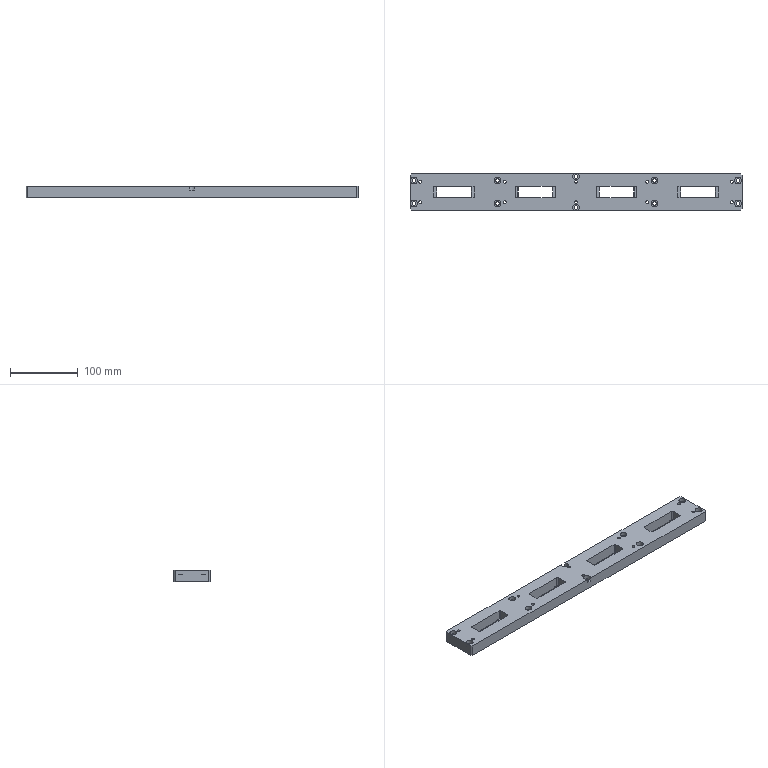NC program | NX | posted with a generic post | part box 490 x 54 x 17 mm
Lines 1858 to 2864 of 8955:
(ZLEVEL_PROFILE_COPY , TOOL : D4)
N3672 T11 M6
N3674 G54
N3676 G17 G0 G90 X449.641 Y-33.2 S8500 M3
N3678 G43 Z30. H11
N3680 Z1.108
N3682 G94 G1 Z-0.392 F1000.
N3684 X449.757 Y-33.4
N3686 G3 X450.103 Y-33.6 R0.4
N3688 G1 X453. F1500.
N3690 Y-30.703
N3692 G3 X452.8 Y-30.357 R0.4
N3694 G1 X452.6 Y-30.241
N3696 Z1.108
N3698 G0 X449.641 Y-33.2 Z0.716
N3700 G1 Z-0.784 F1000.
N3702 X449.757 Y-33.4
N3704 G3 X450.103 Y-33.6 R0.4
N3706 G1 X453. F1500.
N3708 Y-30.703
N3710 G3 X452.8 Y-30.357 R0.4
N3712 G1 X452.6 Y-30.241
N3714 Z0.716
N3716 G0 X449.641 Y-33.2 Z0.324
N3718 G1 Z-1.176 F1000.
N3720 X449.757 Y-33.4
N3722 G3 X450.103 Y-33.6 R0.4
N3724 G1 X453. F1500.
N3726 Y-30.703
N3728 G3 X452.8 Y-30.357 R0.4
N3730 G1 X452.6 Y-30.241
N3732 Z0.324
N3734 G0 X449.641 Y-33.2 Z-0.068
N3736 G1 Z-1.568 F1000.
N3738 X449.757 Y-33.4
N3740 G3 X450.103 Y-33.6 R0.4
N3742 G1 X453. F1500.
N3744 Y-30.703
N3746 G3 X452.8 Y-30.357 R0.4
N3748 G1 X452.6 Y-30.241
N3750 Z-0.068
N3752 G0 X449.641 Y-33.2 Z-0.459
N3754 G1 Z-1.959 F1000.
N3756 X449.757 Y-33.4
N3758 G3 X450.103 Y-33.6 R0.4
N3760 G1 X453. F1500.
N3762 Y-30.703
N3764 G3 X452.8 Y-30.357 R0.4
N3766 G1 X452.6 Y-30.241
N3768 Z-0.459
N3770 G0 X449.641 Y-33.2 Z-0.851
N3772 G1 Z-2.351 F1000.
N3774 X449.757 Y-33.4
N3776 G3 X450.103 Y-33.6 R0.4
N3778 G1 X453. F1500.
N3780 Y-30.703
N3782 G3 X452.8 Y-30.357 R0.4
N3784 G1 X452.6 Y-30.241
N3786 Z-0.851
N3788 G0 X449.641 Y-33.2 Z-1.243
N3790 G1 Z-2.743 F1000.
N3792 X449.757 Y-33.4
N3794 G3 X450.103 Y-33.6 R0.4
N3796 G1 X453. F1500.
N3798 Y-30.703
N3800 G3 X452.8 Y-30.357 R0.4
N3802 G1 X452.6 Y-30.241
N3804 Z-1.243
N3806 G0 X449.641 Y-33.2 Z-1.635
N3808 G1 Z-3.135 F1000.
N3810 X449.757 Y-33.4
N3812 G3 X450.103 Y-33.6 R0.4
N3814 G1 X453. F1500.
N3816 Y-30.703
N3818 G3 X452.8 Y-30.357 R0.4
N3820 G1 X452.6 Y-30.241
N3822 Z-1.635
N3824 G0 X449.641 Y-33.2 Z-2.027
N3826 G1 Z-3.527 F1000.
N3828 X449.757 Y-33.4
N3830 G3 X450.103 Y-33.6 R0.4
N3832 G1 X453. F1500.
N3834 Y-30.703
N3836 G3 X452.8 Y-30.357 R0.4
N3838 G1 X452.6 Y-30.241
N3840 Z-2.027
N3842 G0 X449.641 Y-33.2 Z-2.419
N3844 G1 Z-3.919 F1000.
N3846 X449.757 Y-33.4
N3848 G3 X450.103 Y-33.6 R0.4
N3850 G1 X453. F1500.
N3852 Y-30.703
N3854 G3 X452.8 Y-30.357 R0.4
N3856 G1 X452.6 Y-30.241
N3858 Z-2.419
N3860 G0 X449.641 Y-33.2 Z-2.811
N3862 G1 Z-4.311 F1000.
N3864 X449.757 Y-33.4
N3866 G3 X450.103 Y-33.6 R0.4
N3868 G1 X453. F1500.
N3870 Y-30.703
N3872 G3 X452.8 Y-30.357 R0.4
N3874 G1 X452.6 Y-30.241
N3876 Z-2.811
N3878 G0 X449.641 Y-33.2 Z-3.203
N3880 G1 Z-4.703 F1000.
N3882 X449.757 Y-33.4
N3884 G3 X450.103 Y-33.6 R0.4
N3886 G1 X453. F1500.
N3888 Y-30.703
N3890 G3 X452.8 Y-30.357 R0.4
N3892 G1 X452.6 Y-30.241
N3894 Z-3.203
N3896 G0 X449.641 Y-33.2 Z-3.595
N3898 G1 Z-5.095 F1000.
N3900 X449.757 Y-33.4
N3902 G3 X450.103 Y-33.6 R0.4
N3904 G1 X453. F1500.
N3906 Y-30.703
N3908 G3 X452.8 Y-30.357 R0.4
N3910 G1 X452.6 Y-30.241
N3912 Z-3.595
N3914 G0 X449.641 Y-33.2 Z-3.986
N3916 G1 Z-5.486 F1000.
N3918 X449.757 Y-33.4
N3920 G3 X450.103 Y-33.6 R0.4
N3922 G1 X453. F1500.
N3924 Y-30.703
N3926 G3 X452.8 Y-30.357 R0.4
N3928 G1 X452.6 Y-30.241
N3930 Z-3.986
N3932 G0 X449.641 Y-33.2 Z-4.378
N3934 G1 Z-5.878 F1000.
N3936 X449.757 Y-33.4
N3938 G3 X450.103 Y-33.6 R0.4
N3940 G1 X453. F1500.
N3942 Y-30.703
N3944 G3 X452.8 Y-30.357 R0.4
N3946 G1 X452.6 Y-30.241
N3948 Z-4.378
N3950 G0 X449.641 Y-33.2 Z-4.77
N3952 G1 Z-6.27 F1000.
N3954 X449.757 Y-33.4
N3956 G3 X450.103 Y-33.6 R0.4
N3958 G1 X453. F1500.
N3960 Y-30.703
N3962 G3 X452.8 Y-30.357 R0.4
N3964 G1 X452.6 Y-30.241
N3966 Z-4.77
N3968 G0 X449.641 Y-33.2 Z-5.162
N3970 G1 Z-6.662 F1000.
N3972 X449.757 Y-33.4
N3974 G3 X450.103 Y-33.6 R0.4
N3976 G1 X453. F1500.
N3978 Y-30.703
N3980 G3 X452.8 Y-30.357 R0.4
N3982 G1 X452.6 Y-30.241
N3984 Z-5.162
N3986 G0 X449.641 Y-33.2 Z-5.554
N3988 G1 Z-7.054 F1000.
N3990 X449.757 Y-33.4
N3992 G3 X450.103 Y-33.6 R0.4
N3994 G1 X453. F1500.
N3996 Y-30.703
N3998 G3 X452.8 Y-30.357 R0.4
N4000 G1 X452.6 Y-30.241
N4002 Z-5.554
N4004 G0 X449.641 Y-33.2 Z-5.946
N4006 G1 Z-7.446 F1000.
N4008 X449.757 Y-33.4
N4010 G3 X450.103 Y-33.6 R0.4
N4012 G1 X453. F1500.
N4014 Y-30.703
N4016 G3 X452.8 Y-30.357 R0.4
N4018 G1 X452.6 Y-30.241
N4020 Z-5.946
N4022 G0 X449.641 Y-33.2 Z-6.338
N4024 G1 Z-7.838 F1000.
N4026 X449.757 Y-33.4
N4028 G3 X450.103 Y-33.6 R0.4
N4030 G1 X453. F1500.
N4032 Y-30.703
N4034 G3 X452.8 Y-30.357 R0.4
N4036 G1 X452.6 Y-30.241
N4038 Z-6.338
N4040 G0 X449.641 Y-33.2 Z-6.73
N4042 G1 Z-8.23 F1000.
N4044 X449.757 Y-33.4
N4046 G3 X450.103 Y-33.6 R0.4
N4048 G1 X453. F1500.
N4050 Y-30.703
N4052 G3 X452.8 Y-30.357 R0.4
N4054 G1 X452.6 Y-30.241
N4056 Z-6.73
N4058 G0 X449.641 Y-33.2 Z-7.122
N4060 G1 Z-8.622 F1000.
N4062 X449.757 Y-33.4
N4064 G3 X450.103 Y-33.6 R0.4
N4066 G1 X453. F1500.
N4068 Y-30.703
N4070 G3 X452.8 Y-30.357 R0.4
N4072 G1 X452.6 Y-30.241
N4074 Z-7.122
N4076 G0 X449.641 Y-33.2 Z-7.514
N4078 G1 Z-9.014 F1000.
N4080 X449.757 Y-33.4
N4082 G3 X450.103 Y-33.6 R0.4
N4084 G1 X453. F1500.
N4086 Y-30.703
N4088 G3 X452.8 Y-30.357 R0.4
N4090 G1 X452.6 Y-30.241
N4092 Z-7.514
N4094 G0 X449.641 Y-33.2 Z-7.905
N4096 G1 Z-9.405 F1000.
N4098 X449.757 Y-33.4
N4100 G3 X450.103 Y-33.6 R0.4
N4102 G1 X453. F1500.
N4104 Y-30.703
N4106 G3 X452.8 Y-30.357 R0.4
N4108 G1 X452.6 Y-30.241
N4110 Z-7.905
N4112 G0 X449.641 Y-33.2 Z-8.297
N4114 G1 Z-9.797 F1000.
N4116 X449.757 Y-33.4
N4118 G3 X450.103 Y-33.6 R0.4
N4120 G1 X453. F1500.
N4122 Y-30.703
N4124 G3 X452.8 Y-30.357 R0.4
N4126 G1 X452.6 Y-30.241
N4128 Z-8.297
N4130 G0 X449.641 Y-33.2 Z-8.689
N4132 G1 Z-10.189 F1000.
N4134 X449.757 Y-33.4
N4136 G3 X450.103 Y-33.6 R0.4
N4138 G1 X453. F1500.
N4140 Y-30.703
N4142 G3 X452.8 Y-30.357 R0.4
N4144 G1 X452.6 Y-30.241
N4146 Z-8.689
N4148 G0 X449.641 Y-33.2 Z-9.081
N4150 G1 Z-10.581 F1000.
N4152 X449.757 Y-33.4
N4154 G3 X450.103 Y-33.6 R0.4
N4156 G1 X453. F1500.
N4158 Y-30.703
N4160 G3 X452.8 Y-30.357 R0.4
N4162 G1 X452.6 Y-30.241
N4164 Z-9.081
N4166 G0 X449.641 Y-33.2 Z-9.473
N4168 G1 Z-10.973 F1000.
N4170 X449.757 Y-33.4
N4172 G3 X450.103 Y-33.6 R0.4
N4174 G1 X453. F1500.
N4176 Y-30.703
N4178 G3 X452.8 Y-30.357 R0.4
N4180 G1 X452.6 Y-30.241
N4182 Z-9.473
N4184 G0 X449.641 Y-33.2 Z-9.865
N4186 G1 Z-11.365 F1000.
N4188 X449.757 Y-33.4
N4190 G3 X450.103 Y-33.6 R0.4
N4192 G1 X453. F1500.
N4194 Y-30.703
N4196 G3 X452.8 Y-30.357 R0.4
N4198 G1 X452.6 Y-30.241
N4200 Z-9.865
N4202 G0 X449.641 Y-33.2 Z-10.257
N4204 G1 Z-11.757 F1000.
N4206 X449.757 Y-33.4
N4208 G3 X450.103 Y-33.6 R0.4
N4210 G1 X453. F1500.
N4212 Y-30.703
N4214 G3 X452.8 Y-30.357 R0.4
N4216 G1 X452.6 Y-30.241
N4218 Z-10.257
N4220 G0 X449.641 Y-33.2 Z-10.649
N4222 G1 Z-12.149 F1000.
N4224 X449.757 Y-33.4
N4226 G3 X450.103 Y-33.6 R0.4
N4228 G1 X453. F1500.
N4230 Y-30.703
N4232 G3 X452.8 Y-30.357 R0.4
N4234 G1 X452.6 Y-30.241
N4236 Z-10.649
N4238 G0 X449.641 Y-33.2 Z-11.041
N4240 G1 Z-12.541 F1000.
N4242 X449.757 Y-33.4
N4244 G3 X450.103 Y-33.6 R0.4
N4246 G1 X453. F1500.
N4248 Y-30.703
N4250 G3 X452.8 Y-30.357 R0.4
N4252 G1 X452.6 Y-30.241
N4254 Z-11.041
N4256 G0 X449.641 Y-33.2 Z-11.432
N4258 G1 Z-12.932 F1000.
N4260 X449.757 Y-33.4
N4262 G3 X450.103 Y-33.6 R0.4
N4264 G1 X453. F1500.
N4266 Y-30.703
N4268 G3 X452.8 Y-30.357 R0.4
N4270 G1 X452.6 Y-30.241
N4272 Z-11.432
N4274 G0 X449.641 Y-33.2 Z-11.824
N4276 G1 Z-13.324 F1000.
N4278 X449.757 Y-33.4
N4280 G3 X450.103 Y-33.6 R0.4
N4282 G1 X453. F1500.
N4284 Y-30.703
N4286 G3 X452.8 Y-30.357 R0.4
N4288 G1 X452.6 Y-30.241
N4290 Z-11.824
N4292 G0 X449.641 Y-33.2 Z-12.216
N4294 G1 Z-13.716 F1000.
N4296 X449.757 Y-33.4
N4298 G3 X450.103 Y-33.6 R0.4
N4300 G1 X453. F1500.
N4302 Y-30.703
N4304 G3 X452.8 Y-30.357 R0.4
N4306 G1 X452.6 Y-30.241
N4308 Z-12.216
N4310 G0 X449.641 Y-33.2 Z-12.608
N4312 G1 Z-14.108 F1000.
N4314 X449.757 Y-33.4
N4316 G3 X450.103 Y-33.6 R0.4
N4318 G1 X453. F1500.
N4320 Y-30.703
N4322 G3 X452.8 Y-30.357 R0.4
N4324 G1 X452.6 Y-30.241
N4326 Z-12.608
N4328 G0 X449.641 Y-33.2 Z-13.
N4330 G1 Z-14.5 F1000.
N4332 X449.757 Y-33.4
N4334 G3 X450.103 Y-33.6 R0.4
N4336 G1 X453. F1500.
N4338 Y-30.703
N4340 G3 X452.8 Y-30.357 R0.4
N4342 G1 X452.6 Y-30.241
N4344 Z-13.
N4346 G0 X445.284 Y-33.2 Z-13.357
N4348 G1 Z-14.857 F1000.
N4350 X445.399 Y-33.4
N4352 G3 X445.746 Y-33.6 R0.4
N4354 G1 X448.643 F1500.
N4356 Y-30.703
N4358 G3 X448.443 Y-30.357 R0.4
N4360 G1 X448.243 Y-30.241
N4362 Z-13.357
N4364 G0 X445.141 Y-33.2 Z-13.714
N4366 G1 Z-15.214 F1000.
N4368 X445.257 Y-33.4
N4370 G3 X445.603 Y-33.6 R0.4
N4372 G1 X448.5 F1500.
N4374 Y-30.703
N4376 G3 X448.3 Y-30.357 R0.4
N4378 G1 X448.1 Y-30.241
N4380 Z-13.714
N4382 G0 X445.141 Y-33.2 Z-14.071
N4384 G1 Z-15.571 F1000.
N4386 X445.257 Y-33.4
N4388 G3 X445.603 Y-33.6 R0.4
N4390 G1 X448.5 F1500.
N4392 Y-30.703
N4394 G3 X448.3 Y-30.357 R0.4
N4396 G1 X448.1 Y-30.241
N4398 Z-14.071
N4400 G0 X445.141 Y-33.2 Z-14.429
N4402 G1 Z-15.929 F1000.
N4404 X445.257 Y-33.4
N4406 G3 X445.603 Y-33.6 R0.4
N4408 G1 X448.5 F1500.
N4410 Y-30.703
N4412 G3 X448.3 Y-30.357 R0.4
N4414 G1 X448.1 Y-30.241
N4416 Z-14.429
N4418 G0 X445.138 Y-33.2 Z-14.786
N4420 G1 Z-16.286 F1000.
N4422 X445.254 Y-33.4
N4424 G3 X445.6 Y-33.6 R0.4
N4426 G1 X448.5 F1500.
N4428 Y-30.703
N4430 G3 X448.3 Y-30.356 R0.4
N4432 G1 X448.1 Y-30.241
N4434 Z-14.786
N4436 G0 X445.138 Y-33.2 Z-15.143
N4438 G1 Z-16.643 F1000.
N4440 X445.254 Y-33.4
N4442 G3 X445.6 Y-33.6 R0.4
N4444 G1 X448.5 F1500.
N4446 Y-30.703
N4448 G3 X448.3 Y-30.356 R0.4
N4450 G1 X448.1 Y-30.241
N4452 Z-15.143
N4454 G0 X445.138 Y-33.2 Z-15.5
N4456 G1 Z-17. F1000.
N4458 X445.254 Y-33.4
N4460 G3 X445.6 Y-33.6 R0.4
N4462 G1 X448.5 F1500.
N4464 Y-30.703
N4466 G3 X448.3 Y-30.356 R0.4
N4468 G1 X448.1 Y-30.241
N4470 Z-15.5
N4472 G0 Z30.
N4474 X452.6 Y-23.759
N4476 Z1.108
N4478 G1 Z-0.392 F1000.
N4480 X452.8 Y-23.643
N4482 G3 X453. Y-23.297 R0.4
N4484 G1 Y-20.4 F1500.
N4486 X450.103
N4488 G3 X449.757 Y-20.6 R0.4
N4490 G1 X449.641 Y-20.8
N4492 Z1.108
N4494 G0 X452.6 Y-23.759 Z0.716
N4496 G1 Z-0.784 F1000.
N4498 X452.8 Y-23.643
N4500 G3 X453. Y-23.297 R0.4
N4502 G1 Y-20.4 F1500.
N4504 X450.103
N4506 G3 X449.757 Y-20.6 R0.4
N4508 G1 X449.641 Y-20.8
N4510 Z0.716
N4512 G0 X452.6 Y-23.759 Z0.324
N4514 G1 Z-1.176 F1000.
N4516 X452.8 Y-23.643
N4518 G3 X453. Y-23.297 R0.4
N4520 G1 Y-20.4 F1500.
N4522 X450.103
N4524 G3 X449.757 Y-20.6 R0.4
N4526 G1 X449.641 Y-20.8
N4528 Z0.324
N4530 G0 X452.6 Y-23.759 Z-0.068
N4532 G1 Z-1.568 F1000.
N4534 X452.8 Y-23.643
N4536 G3 X453. Y-23.297 R0.4
N4538 G1 Y-20.4 F1500.
N4540 X450.103
N4542 G3 X449.757 Y-20.6 R0.4
N4544 G1 X449.641 Y-20.8
N4546 Z-0.068
N4548 G0 X452.6 Y-23.759 Z-0.459
N4550 G1 Z-1.959 F1000.
N4552 X452.8 Y-23.643
N4554 G3 X453. Y-23.297 R0.4
N4556 G1 Y-20.4 F1500.
N4558 X450.103
N4560 G3 X449.757 Y-20.6 R0.4
N4562 G1 X449.641 Y-20.8
N4564 Z-0.459
N4566 G0 X452.6 Y-23.759 Z-0.851
N4568 G1 Z-2.351 F1000.
N4570 X452.8 Y-23.643
N4572 G3 X453. Y-23.297 R0.4
N4574 G1 Y-20.4 F1500.
N4576 X450.103
N4578 G3 X449.757 Y-20.6 R0.4
N4580 G1 X449.641 Y-20.8
N4582 Z-0.851
N4584 G0 X452.6 Y-23.759 Z-1.243
N4586 G1 Z-2.743 F1000.
N4588 X452.8 Y-23.643
N4590 G3 X453. Y-23.297 R0.4
N4592 G1 Y-20.4 F1500.
N4594 X450.103
N4596 G3 X449.757 Y-20.6 R0.4
N4598 G1 X449.641 Y-20.8
N4600 Z-1.243
N4602 G0 X452.6 Y-23.759 Z-1.635
N4604 G1 Z-3.135 F1000.
N4606 X452.8 Y-23.643
N4608 G3 X453. Y-23.297 R0.4
N4610 G1 Y-20.4 F1500.
N4612 X450.103
N4614 G3 X449.757 Y-20.6 R0.4
N4616 G1 X449.641 Y-20.8
N4618 Z-1.635
N4620 G0 X452.6 Y-23.759 Z-2.027
N4622 G1 Z-3.527 F1000.
N4624 X452.8 Y-23.643
N4626 G3 X453. Y-23.297 R0.4
N4628 G1 Y-20.4 F1500.
N4630 X450.103
N4632 G3 X449.757 Y-20.6 R0.4
N4634 G1 X449.641 Y-20.8
N4636 Z-2.027
N4638 G0 X452.6 Y-23.759 Z-2.419
N4640 G1 Z-3.919 F1000.
N4642 X452.8 Y-23.643
N4644 G3 X453. Y-23.297 R0.4
N4646 G1 Y-20.4 F1500.
N4648 X450.103
N4650 G3 X449.757 Y-20.6 R0.4
N4652 G1 X449.641 Y-20.8
N4654 Z-2.419
N4656 G0 X452.6 Y-23.759 Z-2.811
N4658 G1 Z-4.311 F1000.
N4660 X452.8 Y-23.643
N4662 G3 X453. Y-23.297 R0.4
N4664 G1 Y-20.4 F1500.
N4666 X450.103
N4668 G3 X449.757 Y-20.6 R0.4
N4670 G1 X449.641 Y-20.8
N4672 Z-2.811
N4674 G0 X452.6 Y-23.759 Z-3.203
N4676 G1 Z-4.703 F1000.
N4678 X452.8 Y-23.643
N4680 G3 X453. Y-23.297 R0.4
N4682 G1 Y-20.4 F1500.
N4684 X450.103
N4686 G3 X449.757 Y-20.6 R0.4
N4688 G1 X449.641 Y-20.8
N4690 Z-3.203
N4692 G0 X452.6 Y-23.759 Z-3.595
N4694 G1 Z-5.095 F1000.
N4696 X452.8 Y-23.643
N4698 G3 X453. Y-23.297 R0.4
N4700 G1 Y-20.4 F1500.
N4702 X450.103
N4704 G3 X449.757 Y-20.6 R0.4
N4706 G1 X449.641 Y-20.8
N4708 Z-3.595
N4710 G0 X452.6 Y-23.759 Z-3.986
N4712 G1 Z-5.486 F1000.
N4714 X452.8 Y-23.643
N4716 G3 X453. Y-23.297 R0.4
N4718 G1 Y-20.4 F1500.
N4720 X450.103
N4722 G3 X449.757 Y-20.6 R0.4
N4724 G1 X449.641 Y-20.8
N4726 Z-3.986
N4728 G0 X452.6 Y-23.759 Z-4.378
N4730 G1 Z-5.878 F1000.
N4732 X452.8 Y-23.643
N4734 G3 X453. Y-23.297 R0.4
N4736 G1 Y-20.4 F1500.
N4738 X450.103
N4740 G3 X449.757 Y-20.6 R0.4
N4742 G1 X449.641 Y-20.8
N4744 Z-4.378
N4746 G0 X452.6 Y-23.759 Z-4.77
N4748 G1 Z-6.27 F1000.
N4750 X452.8 Y-23.643
N4752 G3 X453. Y-23.297 R0.4
N4754 G1 Y-20.4 F1500.
N4756 X450.103
N4758 G3 X449.757 Y-20.6 R0.4
N4760 G1 X449.641 Y-20.8
N4762 Z-4.77
N4764 G0 X452.6 Y-23.759 Z-5.162
N4766 G1 Z-6.662 F1000.
N4768 X452.8 Y-23.643
N4770 G3 X453. Y-23.297 R0.4
N4772 G1 Y-20.4 F1500.
N4774 X450.103
N4776 G3 X449.757 Y-20.6 R0.4
N4778 G1 X449.641 Y-20.8
N4780 Z-5.162
N4782 G0 X452.6 Y-23.759 Z-5.554
N4784 G1 Z-7.054 F1000.
N4786 X452.8 Y-23.643
N4788 G3 X453. Y-23.297 R0.4
N4790 G1 Y-20.4 F1500.
N4792 X450.103
N4794 G3 X449.757 Y-20.6 R0.4
N4796 G1 X449.641 Y-20.8
N4798 Z-5.554
N4800 G0 X452.6 Y-23.759 Z-5.946
N4802 G1 Z-7.446 F1000.
N4804 X452.8 Y-23.643
N4806 G3 X453. Y-23.297 R0.4
N4808 G1 Y-20.4 F1500.
N4810 X450.103
N4812 G3 X449.757 Y-20.6 R0.4
N4814 G1 X449.641 Y-20.8
N4816 Z-5.946
N4818 G0 X452.6 Y-23.759 Z-6.338
N4820 G1 Z-7.838 F1000.
N4822 X452.8 Y-23.643
N4824 G3 X453. Y-23.297 R0.4
N4826 G1 Y-20.4 F1500.
N4828 X450.103
N4830 G3 X449.757 Y-20.6 R0.4
N4832 G1 X449.641 Y-20.8
N4834 Z-6.338
N4836 G0 X452.6 Y-23.759 Z-6.73
N4838 G1 Z-8.23 F1000.
N4840 X452.8 Y-23.643
N4842 G3 X453. Y-23.297 R0.4
N4844 G1 Y-20.4 F1500.
N4846 X450.103
N4848 G3 X449.757 Y-20.6 R0.4
N4850 G1 X449.641 Y-20.8
N4852 Z-6.73
N4854 G0 X452.6 Y-23.759 Z-7.122
N4856 G1 Z-8.622 F1000.
N4858 X452.8 Y-23.643
N4860 G3 X453. Y-23.297 R0.4
N4862 G1 Y-20.4 F1500.
N4864 X450.103
N4866 G3 X449.757 Y-20.6 R0.4
N4868 G1 X449.641 Y-20.8
N4870 Z-7.122
N4872 G0 X452.6 Y-23.759 Z-7.514
N4874 G1 Z-9.014 F1000.
N4876 X452.8 Y-23.643
N4878 G3 X453. Y-23.297 R0.4
N4880 G1 Y-20.4 F1500.
N4882 X450.103
N4884 G3 X449.757 Y-20.6 R0.4
N4886 G1 X449.641 Y-20.8
N4888 Z-7.514
N4890 G0 X452.6 Y-23.759 Z-7.905
N4892 G1 Z-9.405 F1000.
N4894 X452.8 Y-23.643
N4896 G3 X453. Y-23.297 R0.4
N4898 G1 Y-20.4 F1500.
N4900 X450.103
N4902 G3 X449.757 Y-20.6 R0.4
N4904 G1 X449.641 Y-20.8
N4906 Z-7.905
N4908 G0 X452.6 Y-23.759 Z-8.297
N4910 G1 Z-9.797 F1000.
N4912 X452.8 Y-23.643
N4914 G3 X453. Y-23.297 R0.4
N4916 G1 Y-20.4 F1500.
N4918 X450.103
N4920 G3 X449.757 Y-20.6 R0.4
N4922 G1 X449.641 Y-20.8
N4924 Z-8.297
N4926 G0 X452.6 Y-23.759 Z-8.689
N4928 G1 Z-10.189 F1000.
N4930 X452.8 Y-23.643
N4932 G3 X453. Y-23.297 R0.4
N4934 G1 Y-20.4 F1500.
N4936 X450.103
N4938 G3 X449.757 Y-20.6 R0.4
N4940 G1 X449.641 Y-20.8
N4942 Z-8.689
N4944 G0 X452.6 Y-23.759 Z-9.081
N4946 G1 Z-10.581 F1000.
N4948 X452.8 Y-23.643
N4950 G3 X453. Y-23.297 R0.4
N4952 G1 Y-20.4 F1500.
N4954 X450.103
N4956 G3 X449.757 Y-20.6 R0.4
N4958 G1 X449.641 Y-20.8
N4960 Z-9.081
N4962 G0 X452.6 Y-23.759 Z-9.473
N4964 G1 Z-10.973 F1000.
N4966 X452.8 Y-23.643
N4968 G3 X453. Y-23.297 R0.4
N4970 G1 Y-20.4 F1500.
N4972 X450.103
N4974 G3 X449.757 Y-20.6 R0.4
N4976 G1 X449.641 Y-20.8
N4978 Z-9.473
N4980 G0 X452.6 Y-23.759 Z-9.865
N4982 G1 Z-11.365 F1000.
N4984 X452.8 Y-23.643
N4986 G3 X453. Y-23.297 R0.4
N4988 G1 Y-20.4 F1500.
N4990 X450.103
N4992 G3 X449.757 Y-20.6 R0.4
N4994 G1 X449.641 Y-20.8
N4996 Z-9.865
N4998 G0 X452.6 Y-23.759 Z-10.257
N5000 G1 Z-11.757 F1000.
N5002 X452.8 Y-23.643
N5004 G3 X453. Y-23.297 R0.4
N5006 G1 Y-20.4 F1500.
N5008 X450.103
N5010 G3 X449.757 Y-20.6 R0.4
N5012 G1 X449.641 Y-20.8
N5014 Z-10.257
N5016 G0 X452.6 Y-23.759 Z-10.649
N5018 G1 Z-12.149 F1000.
N5020 X452.8 Y-23.643
N5022 G3 X453. Y-23.297 R0.4
N5024 G1 Y-20.4 F1500.
N5026 X450.103
N5028 G3 X449.757 Y-20.6 R0.4
N5030 G1 X449.641 Y-20.8
N5032 Z-10.649
N5034 G0 X452.6 Y-23.759 Z-11.041
N5036 G1 Z-12.541 F1000.
N5038 X452.8 Y-23.643
N5040 G3 X453. Y-23.297 R0.4
N5042 G1 Y-20.4 F1500.
N5044 X450.103
N5046 G3 X449.757 Y-20.6 R0.4
N5048 G1 X449.641 Y-20.8
N5050 Z-11.041
N5052 G0 X452.6 Y-23.759 Z-11.432
N5054 G1 Z-12.932 F1000.
N5056 X452.8 Y-23.643
N5058 G3 X453. Y-23.297 R0.4
N5060 G1 Y-20.4 F1500.
N5062 X450.103
N5064 G3 X449.757 Y-20.6 R0.4
N5066 G1 X449.641 Y-20.8
N5068 Z-11.432
N5070 G0 X452.6 Y-23.759 Z-11.824
N5072 G1 Z-13.324 F1000.
N5074 X452.8 Y-23.643
N5076 G3 X453. Y-23.297 R0.4
N5078 G1 Y-20.4 F1500.
N5080 X450.103
N5082 G3 X449.757 Y-20.6 R0.4
N5084 G1 X449.641 Y-20.8
N5086 Z-11.824
N5088 G0 X452.6 Y-23.759 Z-12.216
N5090 G1 Z-13.716 F1000.
N5092 X452.8 Y-23.643
N5094 G3 X453. Y-23.297 R0.4
N5096 G1 Y-20.4 F1500.
N5098 X450.103
N5100 G3 X449.757 Y-20.6 R0.4
N5102 G1 X449.641 Y-20.8
N5104 Z-12.216
N5106 G0 X452.6 Y-23.759 Z-12.608
N5108 G1 Z-14.108 F1000.
N5110 X452.8 Y-23.643
N5112 G3 X453. Y-23.297 R0.4
N5114 G1 Y-20.4 F1500.
N5116 X450.103
N5118 G3 X449.757 Y-20.6 R0.4
N5120 G1 X449.641 Y-20.8
N5122 Z-12.608
N5124 G0 X452.6 Y-23.759 Z-13.
N5126 G1 Z-14.5 F1000.
N5128 X452.8 Y-23.643
N5130 G3 X453. Y-23.297 R0.4
N5132 G1 Y-20.4 F1500.
N5134 X450.103
N5136 G3 X449.757 Y-20.6 R0.4
N5138 G1 X449.641 Y-20.8
N5140 Z-13.
N5142 G0 X448.243 Y-23.759 Z-13.357
N5144 G1 Z-14.857 F1000.
N5146 X448.443 Y-23.643
N5148 G3 X448.643 Y-23.297 R0.4
N5150 G1 Y-20.4 F1500.
N5152 X445.746
N5154 G3 X445.399 Y-20.6 R0.4
N5156 G1 X445.284 Y-20.8
N5158 Z-13.357
N5160 G0 X448.1 Y-23.759 Z-13.714
N5162 G1 Z-15.214 F1000.
N5164 X448.3 Y-23.643
N5166 G3 X448.5 Y-23.297 R0.4
N5168 G1 Y-20.4 F1500.
N5170 X445.603
N5172 G3 X445.257 Y-20.6 R0.4
N5174 G1 X445.141 Y-20.8
N5176 Z-13.714
N5178 G0 X448.1 Y-23.759 Z-14.071
N5180 G1 Z-15.571 F1000.
N5182 X448.3 Y-23.643
N5184 G3 X448.5 Y-23.297 R0.4
N5186 G1 Y-20.4 F1500.
N5188 X445.603
N5190 G3 X445.257 Y-20.6 R0.4
N5192 G1 X445.141 Y-20.8
N5194 Z-14.071
N5196 G0 X448.1 Y-23.759 Z-14.429
N5198 G1 Z-15.929 F1000.
N5200 X448.3 Y-23.643
N5202 G3 X448.5 Y-23.297 R0.4
N5204 G1 Y-20.4 F1500.
N5206 X445.603
N5208 G3 X445.257 Y-20.6 R0.4
N5210 G1 X445.141 Y-20.8
N5212 Z-14.429
N5214 G0 X448.1 Y-23.759 Z-14.786
N5216 G1 Z-16.286 F1000.
N5218 X448.3 Y-23.644
N5220 G3 X448.5 Y-23.297 R0.4
N5222 G1 Y-20.4 F1500.
N5224 X445.6
N5226 G3 X445.254 Y-20.6 R0.4
N5228 G1 X445.138 Y-20.8
N5230 Z-14.786
N5232 G0 X448.1 Y-23.759 Z-15.143
N5234 G1 Z-16.643 F1000.
N5236 X448.3 Y-23.644
N5238 G3 X448.5 Y-23.297 R0.4
N5240 G1 Y-20.4 F1500.
N5242 X445.6
N5244 G3 X445.254 Y-20.6 R0.4
N5246 G1 X445.138 Y-20.8
N5248 Z-15.143
N5250 G0 X448.1 Y-23.759 Z-15.5
N5252 G1 Z-17. F1000.
N5254 X448.3 Y-23.644
N5256 G3 X448.5 Y-23.297 R0.4
N5258 G1 Y-20.4 F1500.
N5260 X445.6
N5262 G3 X445.254 Y-20.6 R0.4
N5264 G1 X445.138 Y-20.8
N5266 Z-15.5
N5268 G0 Z30.
N5270 X400.359
N5272 Z1.108
N5274 G1 Z-0.392 F1000.
N5276 X400.243 Y-20.6
N5278 G3 X399.897 Y-20.4 R0.4
N5280 G1 X397. F1500.
N5282 Y-23.297
N5284 G3 X397.2 Y-23.643 R0.4
N5286 G1 X397.4 Y-23.759
N5288 Z1.108
N5290 G0 X400.359 Y-20.8 Z0.716
N5292 G1 Z-0.784 F1000.
N5294 X400.243 Y-20.6
N5296 G3 X399.897 Y-20.4 R0.4
N5298 G1 X397. F1500.
N5300 Y-23.297
N5302 G3 X397.2 Y-23.643 R0.4
N5304 G1 X397.4 Y-23.759
N5306 Z0.716
N5308 G0 X400.359 Y-20.8 Z0.324
N5310 G1 Z-1.176 F1000.
N5312 X400.243 Y-20.6
N5314 G3 X399.897 Y-20.4 R0.4
N5316 G1 X397. F1500.
N5318 Y-23.297
N5320 G3 X397.2 Y-23.643 R0.4
N5322 G1 X397.4 Y-23.759
N5324 Z0.324
N5326 G0 X400.359 Y-20.8 Z-0.068
N5328 G1 Z-1.568 F1000.
N5330 X400.243 Y-20.6
N5332 G3 X399.897 Y-20.4 R0.4
N5334 G1 X397. F1500.
N5336 Y-23.297
N5338 G3 X397.2 Y-23.643 R0.4
N5340 G1 X397.4 Y-23.759
N5342 Z-0.068
N5344 G0 X400.359 Y-20.8 Z-0.459
N5346 G1 Z-1.959 F1000.
N5348 X400.243 Y-20.6
N5350 G3 X399.897 Y-20.4 R0.4
N5352 G1 X397. F1500.
N5354 Y-23.297
N5356 G3 X397.2 Y-23.643 R0.4
N5358 G1 X397.4 Y-23.759
N5360 Z-0.459
N5362 G0 X400.359 Y-20.8 Z-0.851
N5364 G1 Z-2.351 F1000.
N5366 X400.243 Y-20.6
N5368 G3 X399.897 Y-20.4 R0.4
N5370 G1 X397. F1500.
N5372 Y-23.297
N5374 G3 X397.2 Y-23.643 R0.4
N5376 G1 X397.4 Y-23.759
N5378 Z-0.851
N5380 G0 X400.359 Y-20.8 Z-1.243
N5382 G1 Z-2.743 F1000.
N5384 X400.243 Y-20.6
N5386 G3 X399.897 Y-20.4 R0.4
N5388 G1 X397. F1500.
N5390 Y-23.297
N5392 G3 X397.2 Y-23.643 R0.4
N5394 G1 X397.4 Y-23.759
N5396 Z-1.243
N5398 G0 X400.359 Y-20.8 Z-1.635
N5400 G1 Z-3.135 F1000.
N5402 X400.243 Y-20.6
N5404 G3 X399.897 Y-20.4 R0.4
N5406 G1 X397. F1500.
N5408 Y-23.297
N5410 G3 X397.2 Y-23.643 R0.4
N5412 G1 X397.4 Y-23.759
N5414 Z-1.635
N5416 G0 X400.359 Y-20.8 Z-2.027
N5418 G1 Z-3.527 F1000.
N5420 X400.243 Y-20.6
N5422 G3 X399.897 Y-20.4 R0.4
N5424 G1 X397. F1500.
N5426 Y-23.297
N5428 G3 X397.2 Y-23.643 R0.4
N5430 G1 X397.4 Y-23.759
N5432 Z-2.027
N5434 G0 X400.359 Y-20.8 Z-2.419
N5436 G1 Z-3.919 F1000.
N5438 X400.243 Y-20.6
N5440 G3 X399.897 Y-20.4 R0.4
N5442 G1 X397. F1500.
N5444 Y-23.297
N5446 G3 X397.2 Y-23.643 R0.4
N5448 G1 X397.4 Y-23.759
N5450 Z-2.419
N5452 G0 X400.359 Y-20.8 Z-2.811
N5454 G1 Z-4.311 F1000.
N5456 X400.243 Y-20.6
N5458 G3 X399.897 Y-20.4 R0.4
N5460 G1 X397. F1500.
N5462 Y-23.297
N5464 G3 X397.2 Y-23.643 R0.4
N5466 G1 X397.4 Y-23.759
N5468 Z-2.811
N5470 G0 X400.359 Y-20.8 Z-3.203
N5472 G1 Z-4.703 F1000.
N5474 X400.243 Y-20.6
N5476 G3 X399.897 Y-20.4 R0.4
N5478 G1 X397. F1500.
N5480 Y-23.297
N5482 G3 X397.2 Y-23.643 R0.4
N5484 G1 X397.4 Y-23.759
N5486 Z-3.203
N5488 G0 X400.359 Y-20.8 Z-3.595
N5490 G1 Z-5.095 F1000.
N5492 X400.243 Y-20.6
N5494 G3 X399.897 Y-20.4 R0.4
N5496 G1 X397. F1500.
N5498 Y-23.297
N5500 G3 X397.2 Y-23.643 R0.4
N5502 G1 X397.4 Y-23.759
N5504 Z-3.595
N5506 G0 X400.359 Y-20.8 Z-3.986
N5508 G1 Z-5.486 F1000.
N5510 X400.243 Y-20.6
N5512 G3 X399.897 Y-20.4 R0.4
N5514 G1 X397. F1500.
N5516 Y-23.297
N5518 G3 X397.2 Y-23.643 R0.4
N5520 G1 X397.4 Y-23.759
N5522 Z-3.986
N5524 G0 X400.359 Y-20.8 Z-4.378
N5526 G1 Z-5.878 F1000.
N5528 X400.243 Y-20.6
N5530 G3 X399.897 Y-20.4 R0.4
N5532 G1 X397. F1500.
N5534 Y-23.297
N5536 G3 X397.2 Y-23.643 R0.4
N5538 G1 X397.4 Y-23.759
N5540 Z-4.378
N5542 G0 X400.359 Y-20.8 Z-4.77
N5544 G1 Z-6.27 F1000.
N5546 X400.243 Y-20.6
N5548 G3 X399.897 Y-20.4 R0.4
N5550 G1 X397. F1500.
N5552 Y-23.297
N5554 G3 X397.2 Y-23.643 R0.4
N5556 G1 X397.4 Y-23.759
N5558 Z-4.77
N5560 G0 X400.359 Y-20.8 Z-5.162
N5562 G1 Z-6.662 F1000.
N5564 X400.243 Y-20.6
N5566 G3 X399.897 Y-20.4 R0.4
N5568 G1 X397. F1500.
N5570 Y-23.297
N5572 G3 X397.2 Y-23.643 R0.4
N5574 G1 X397.4 Y-23.759
N5576 Z-5.162
N5578 G0 X400.359 Y-20.8 Z-5.554
N5580 G1 Z-7.054 F1000.
N5582 X400.243 Y-20.6
N5584 G3 X399.897 Y-20.4 R0.4
N5586 G1 X397. F1500.
N5588 Y-23.297
N5590 G3 X397.2 Y-23.643 R0.4
N5592 G1 X397.4 Y-23.759
N5594 Z-5.554
N5596 G0 X400.359 Y-20.8 Z-5.946
N5598 G1 Z-7.446 F1000.
N5600 X400.243 Y-20.6
N5602 G3 X399.897 Y-20.4 R0.4
N5604 G1 X397. F1500.
N5606 Y-23.297
N5608 G3 X397.2 Y-23.643 R0.4
N5610 G1 X397.4 Y-23.759
N5612 Z-5.946
N5614 G0 X400.359 Y-20.8 Z-6.338
N5616 G1 Z-7.838 F1000.
N5618 X400.243 Y-20.6
N5620 G3 X399.897 Y-20.4 R0.4
N5622 G1 X397. F1500.
N5624 Y-23.297
N5626 G3 X397.2 Y-23.643 R0.4
N5628 G1 X397.4 Y-23.759
N5630 Z-6.338
N5632 G0 X400.359 Y-20.8 Z-6.73
N5634 G1 Z-8.23 F1000.
N5636 X400.243 Y-20.6
N5638 G3 X399.897 Y-20.4 R0.4
N5640 G1 X397. F1500.
N5642 Y-23.297
N5644 G3 X397.2 Y-23.643 R0.4
N5646 G1 X397.4 Y-23.759
N5648 Z-6.73
N5650 G0 X400.359 Y-20.8 Z-7.122
N5652 G1 Z-8.622 F1000.
N5654 X400.243 Y-20.6
N5656 G3 X399.897 Y-20.4 R0.4
N5658 G1 X397. F1500.
N5660 Y-23.297
N5662 G3 X397.2 Y-23.643 R0.4
N5664 G1 X397.4 Y-23.759
N5666 Z-7.122
N5668 G0 X400.359 Y-20.8 Z-7.514
N5670 G1 Z-9.014 F1000.
N5672 X400.243 Y-20.6
N5674 G3 X399.897 Y-20.4 R0.4
N5676 G1 X397. F1500.
N5678 Y-23.297